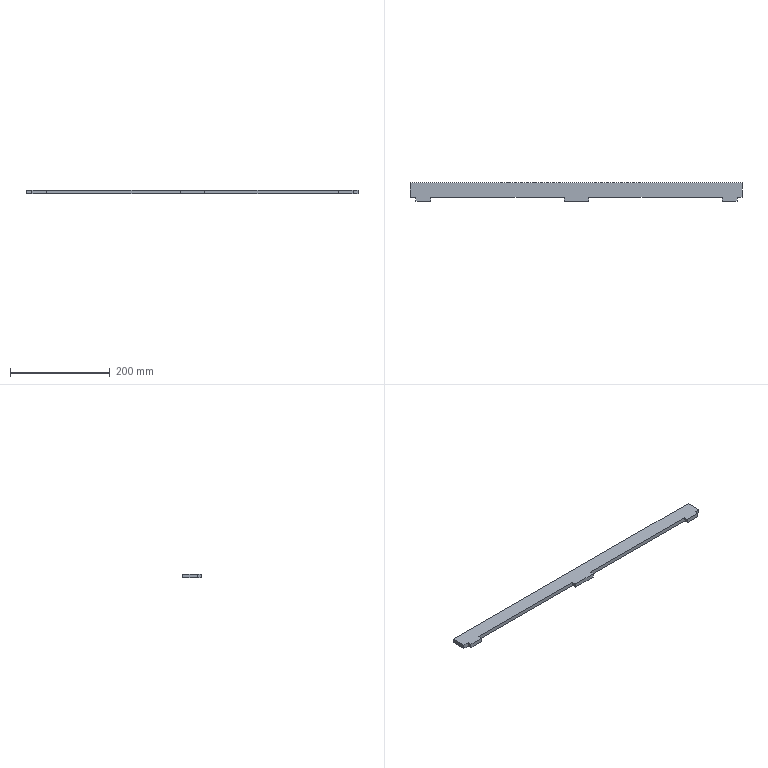Part | SolidWorks | features FlatPattern 1, ICE 1, SMBaseFlange 1, SheetMetal 1 | 1 solid | 18 faces | box 667 x 38 x 8 mm | volume 167120 mm3 | plane 18
STEP:
#1=CARTESIAN_POINT('',(332.5,-15.,-8.));
#2=VERTEX_POINT('',#1);
#3=CARTESIAN_POINT('',(332.5,-15.,0.));
#4=VERTEX_POINT('',#3);
#5=CARTESIAN_POINT('',(332.5,-15.,-8.));
#6=DIRECTION('',(0.,0.,1.));
#7=VECTOR('',#6,1000.);
#8=LINE('',#5,#7);
#9=EDGE_CURVE('',#2,#4,#8,.T.);
#10=ORIENTED_EDGE('',*,*,#9,.T.);
#11=CARTESIAN_POINT('',(322.5,-15.,0.));
#12=VERTEX_POINT('',#11);
#13=CARTESIAN_POINT('',(322.5,-15.,0.));
#14=DIRECTION('',(1.,0.,0.));
#15=VECTOR('',#14,1000.);
#16=LINE('',#13,#15);
#17=EDGE_CURVE('',#12,#4,#16,.T.);
#18=ORIENTED_EDGE('',*,*,#17,.F.);
#19=CARTESIAN_POINT('',(322.5,-15.,-8.));
#20=VERTEX_POINT('',#19);
#21=CARTESIAN_POINT('',(322.5,-15.,-8.));
#22=DIRECTION('',(0.,0.,1.));
#23=VECTOR('',#22,1000.);
#24=LINE('',#21,#23);
#25=EDGE_CURVE('',#20,#12,#24,.T.);
#26=ORIENTED_EDGE('',*,*,#25,.F.);
#27=CARTESIAN_POINT('',(322.5,-15.,-8.));
#28=DIRECTION('',(1.,0.,0.));
#29=VECTOR('',#28,1000.);
#30=LINE('',#27,#29);
#31=EDGE_CURVE('',#20,#2,#30,.T.);
#32=ORIENTED_EDGE('',*,*,#31,.T.);
#33=EDGE_LOOP('',(#10,#18,#26,#32));
#34=FACE_OUTER_BOUND('',#33,.T.);
#35=CARTESIAN_POINT('',(322.5,-15.,-8.));
#36=DIRECTION('',(0.,-1.,0.));
#37=DIRECTION('',(1.,0.,0.));
#38=AXIS2_PLACEMENT_3D('',#35,#36,#37);
#39=PLANE('',#38);
#40=ADVANCED_FACE('',(#34),#39,.T.);
#41=CARTESIAN_POINT('',(322.5,-23.,0.));
#42=VERTEX_POINT('',#41);
#43=CARTESIAN_POINT('',(322.5,-15.,0.));
#44=DIRECTION('',(0.,1.,0.));
#45=VECTOR('',#44,1000.);
#46=LINE('',#43,#45);
#47=EDGE_CURVE('',#42,#12,#46,.T.);
#48=ORIENTED_EDGE('',*,*,#47,.F.);
#49=CARTESIAN_POINT('',(322.5,-23.,-8.));
#50=VERTEX_POINT('',#49);
#51=CARTESIAN_POINT('',(322.5,-23.,-8.));
#52=DIRECTION('',(0.,0.,1.));
#53=VECTOR('',#52,1000.);
#54=LINE('',#51,#53);
#55=EDGE_CURVE('',#50,#42,#54,.T.);
#56=ORIENTED_EDGE('',*,*,#55,.F.);
#57=CARTESIAN_POINT('',(322.5,-15.,-8.));
#58=DIRECTION('',(0.,1.,0.));
#59=VECTOR('',#58,1000.);
#60=LINE('',#57,#59);
#61=EDGE_CURVE('',#50,#20,#60,.T.);
#62=ORIENTED_EDGE('',*,*,#61,.T.);
#63=ORIENTED_EDGE('',*,*,#25,.T.);
#64=EDGE_LOOP('',(#48,#56,#62,#63));
#65=FACE_OUTER_BOUND('',#64,.T.);
#66=CARTESIAN_POINT('',(322.5,-15.,-8.));
#67=DIRECTION('',(1.,0.,0.));
#68=DIRECTION('',(0.,0.,-1.));
#69=AXIS2_PLACEMENT_3D('',#66,#67,#68);
#70=PLANE('',#69);
#71=ADVANCED_FACE('',(#65),#70,.T.);
#72=CARTESIAN_POINT('',(292.5,-23.,0.));
#73=VERTEX_POINT('',#72);
#74=CARTESIAN_POINT('',(322.5,-23.,0.));
#75=DIRECTION('',(1.,0.,0.));
#76=VECTOR('',#75,1000.);
#77=LINE('',#74,#76);
#78=EDGE_CURVE('',#73,#42,#77,.T.);
#79=ORIENTED_EDGE('',*,*,#78,.F.);
#80=CARTESIAN_POINT('',(292.5,-23.,-8.));
#81=VERTEX_POINT('',#80);
#82=CARTESIAN_POINT('',(292.5,-23.,-8.));
#83=DIRECTION('',(0.,0.,1.));
#84=VECTOR('',#83,1000.);
#85=LINE('',#82,#84);
#86=EDGE_CURVE('',#81,#73,#85,.T.);
#87=ORIENTED_EDGE('',*,*,#86,.F.);
#88=CARTESIAN_POINT('',(322.5,-23.,-8.));
#89=DIRECTION('',(1.,0.,0.));
#90=VECTOR('',#89,1000.);
#91=LINE('',#88,#90);
#92=EDGE_CURVE('',#81,#50,#91,.T.);
#93=ORIENTED_EDGE('',*,*,#92,.T.);
#94=ORIENTED_EDGE('',*,*,#55,.T.);
#95=EDGE_LOOP('',(#79,#87,#93,#94));
#96=FACE_OUTER_BOUND('',#95,.T.);
#97=CARTESIAN_POINT('',(322.5,-23.,-8.));
#98=DIRECTION('',(0.,-1.,0.));
#99=DIRECTION('',(1.,0.,0.));
#100=AXIS2_PLACEMENT_3D('',#97,#98,#99);
#101=PLANE('',#100);
#102=ADVANCED_FACE('',(#96),#101,.T.);
#103=CARTESIAN_POINT('',(292.5,-15.,0.));
#104=VERTEX_POINT('',#103);
#105=CARTESIAN_POINT('',(292.5,-23.,0.));
#106=DIRECTION('',(0.,-1.,0.));
#107=VECTOR('',#106,1000.);
#108=LINE('',#105,#107);
#109=EDGE_CURVE('',#104,#73,#108,.T.);
#110=ORIENTED_EDGE('',*,*,#109,.F.);
#111=CARTESIAN_POINT('',(292.5,-15.,-8.));
#112=VERTEX_POINT('',#111);
#113=CARTESIAN_POINT('',(292.5,-15.,-8.));
#114=DIRECTION('',(0.,0.,1.));
#115=VECTOR('',#114,1000.);
#116=LINE('',#113,#115);
#117=EDGE_CURVE('',#112,#104,#116,.T.);
#118=ORIENTED_EDGE('',*,*,#117,.F.);
#119=CARTESIAN_POINT('',(292.5,-23.,-8.));
#120=DIRECTION('',(0.,-1.,0.));
#121=VECTOR('',#120,1000.);
#122=LINE('',#119,#121);
#123=EDGE_CURVE('',#112,#81,#122,.T.);
#124=ORIENTED_EDGE('',*,*,#123,.T.);
#125=ORIENTED_EDGE('',*,*,#86,.T.);
#126=EDGE_LOOP('',(#110,#118,#124,#125));
#127=FACE_OUTER_BOUND('',#126,.T.);
#128=CARTESIAN_POINT('',(292.5,-23.,-8.));
#129=DIRECTION('',(-1.,0.,0.));
#130=DIRECTION('',(0.,0.,1.));
#131=AXIS2_PLACEMENT_3D('',#128,#129,#130);
#132=PLANE('',#131);
#133=ADVANCED_FACE('',(#127),#132,.T.);
#134=CARTESIAN_POINT('',(25.,-15.,0.));
#135=VERTEX_POINT('',#134);
#136=CARTESIAN_POINT('',(25.,-15.,0.));
#137=DIRECTION('',(1.,0.,0.));
#138=VECTOR('',#137,1000.);
#139=LINE('',#136,#138);
#140=EDGE_CURVE('',#135,#104,#139,.T.);
#141=ORIENTED_EDGE('',*,*,#140,.F.);
#142=CARTESIAN_POINT('',(25.,-15.,-8.));
#143=VERTEX_POINT('',#142);
#144=CARTESIAN_POINT('',(25.,-15.,-8.));
#145=DIRECTION('',(0.,0.,1.));
#146=VECTOR('',#145,1000.);
#147=LINE('',#144,#146);
#148=EDGE_CURVE('',#143,#135,#147,.T.);
#149=ORIENTED_EDGE('',*,*,#148,.F.);
#150=CARTESIAN_POINT('',(25.,-15.,-8.));
#151=DIRECTION('',(1.,0.,0.));
#152=VECTOR('',#151,1000.);
#153=LINE('',#150,#152);
#154=EDGE_CURVE('',#143,#112,#153,.T.);
#155=ORIENTED_EDGE('',*,*,#154,.T.);
#156=ORIENTED_EDGE('',*,*,#117,.T.);
#157=EDGE_LOOP('',(#141,#149,#155,#156));
#158=FACE_OUTER_BOUND('',#157,.T.);
#159=CARTESIAN_POINT('',(25.,-15.,-8.));
#160=DIRECTION('',(0.,-1.,0.));
#161=DIRECTION('',(1.,0.,0.));
#162=AXIS2_PLACEMENT_3D('',#159,#160,#161);
#163=PLANE('',#162);
#164=ADVANCED_FACE('',(#158),#163,.T.);
#165=CARTESIAN_POINT('',(25.,-23.,0.));
#166=VERTEX_POINT('',#165);
#167=CARTESIAN_POINT('',(25.,-23.,0.));
#168=DIRECTION('',(0.,1.,0.));
#169=VECTOR('',#168,1000.);
#170=LINE('',#167,#169);
#171=EDGE_CURVE('',#166,#135,#170,.T.);
#172=ORIENTED_EDGE('',*,*,#171,.F.);
#173=CARTESIAN_POINT('',(25.,-23.,-8.));
#174=VERTEX_POINT('',#173);
#175=CARTESIAN_POINT('',(25.,-23.,-8.));
#176=DIRECTION('',(0.,0.,1.));
#177=VECTOR('',#176,1000.);
#178=LINE('',#175,#177);
#179=EDGE_CURVE('',#174,#166,#178,.T.);
#180=ORIENTED_EDGE('',*,*,#179,.F.);
#181=CARTESIAN_POINT('',(25.,-23.,-8.));
#182=DIRECTION('',(0.,1.,0.));
#183=VECTOR('',#182,1000.);
#184=LINE('',#181,#183);
#185=EDGE_CURVE('',#174,#143,#184,.T.);
#186=ORIENTED_EDGE('',*,*,#185,.T.);
#187=ORIENTED_EDGE('',*,*,#148,.T.);
#188=EDGE_LOOP('',(#172,#180,#186,#187));
#189=FACE_OUTER_BOUND('',#188,.T.);
#190=CARTESIAN_POINT('',(25.,-23.,-8.));
#191=DIRECTION('',(1.,0.,0.));
#192=DIRECTION('',(0.,0.,-1.));
#193=AXIS2_PLACEMENT_3D('',#190,#191,#192);
#194=PLANE('',#193);
#195=ADVANCED_FACE('',(#189),#194,.T.);
#196=CARTESIAN_POINT('',(-25.,-23.,0.));
#197=VERTEX_POINT('',#196);
#198=CARTESIAN_POINT('',(-25.,-23.,0.));
#199=DIRECTION('',(1.,0.,0.));
#200=VECTOR('',#199,1000.);
#201=LINE('',#198,#200);
#202=EDGE_CURVE('',#197,#166,#201,.T.);
#203=ORIENTED_EDGE('',*,*,#202,.F.);
#204=CARTESIAN_POINT('',(-25.,-23.,-8.));
#205=VERTEX_POINT('',#204);
#206=CARTESIAN_POINT('',(-25.,-23.,-8.));
#207=DIRECTION('',(0.,0.,1.));
#208=VECTOR('',#207,1000.);
#209=LINE('',#206,#208);
#210=EDGE_CURVE('',#205,#197,#209,.T.);
#211=ORIENTED_EDGE('',*,*,#210,.F.);
#212=CARTESIAN_POINT('',(-25.,-23.,-8.));
#213=DIRECTION('',(1.,0.,0.));
#214=VECTOR('',#213,1000.);
#215=LINE('',#212,#214);
#216=EDGE_CURVE('',#205,#174,#215,.T.);
#217=ORIENTED_EDGE('',*,*,#216,.T.);
#218=ORIENTED_EDGE('',*,*,#179,.T.);
#219=EDGE_LOOP('',(#203,#211,#217,#218));
#220=FACE_OUTER_BOUND('',#219,.T.);
#221=CARTESIAN_POINT('',(-25.,-23.,-8.));
#222=DIRECTION('',(0.,-1.,0.));
#223=DIRECTION('',(1.,0.,0.));
#224=AXIS2_PLACEMENT_3D('',#221,#222,#223);
#225=PLANE('',#224);
#226=ADVANCED_FACE('',(#220),#225,.T.);
#227=CARTESIAN_POINT('',(-25.,-15.,0.));
#228=VERTEX_POINT('',#227);
#229=CARTESIAN_POINT('',(-25.,-15.,0.));
#230=DIRECTION('',(0.,-1.,0.));
#231=VECTOR('',#230,1000.);
#232=LINE('',#229,#231);
#233=EDGE_CURVE('',#228,#197,#232,.T.);
#234=ORIENTED_EDGE('',*,*,#233,.F.);
#235=CARTESIAN_POINT('',(-25.,-15.,-8.));
#236=VERTEX_POINT('',#235);
#237=CARTESIAN_POINT('',(-25.,-15.,-8.));
#238=DIRECTION('',(0.,0.,1.));
#239=VECTOR('',#238,1000.);
#240=LINE('',#237,#239);
#241=EDGE_CURVE('',#236,#228,#240,.T.);
#242=ORIENTED_EDGE('',*,*,#241,.F.);
#243=CARTESIAN_POINT('',(-25.,-15.,-8.));
#244=DIRECTION('',(0.,-1.,0.));
#245=VECTOR('',#244,1000.);
#246=LINE('',#243,#245);
#247=EDGE_CURVE('',#236,#205,#246,.T.);
#248=ORIENTED_EDGE('',*,*,#247,.T.);
#249=ORIENTED_EDGE('',*,*,#210,.T.);
#250=EDGE_LOOP('',(#234,#242,#248,#249));
#251=FACE_OUTER_BOUND('',#250,.T.);
#252=CARTESIAN_POINT('',(-25.,-15.,-8.));
#253=DIRECTION('',(-1.,0.,0.));
#254=DIRECTION('',(0.,0.,1.));
#255=AXIS2_PLACEMENT_3D('',#252,#253,#254);
#256=PLANE('',#255);
#257=ADVANCED_FACE('',(#251),#256,.T.);
#258=CARTESIAN_POINT('',(-292.5,-15.,0.));
#259=VERTEX_POINT('',#258);
#260=CARTESIAN_POINT('',(-292.5,-15.,0.));
#261=DIRECTION('',(1.,0.,0.));
#262=VECTOR('',#261,1000.);
#263=LINE('',#260,#262);
#264=EDGE_CURVE('',#259,#228,#263,.T.);
#265=ORIENTED_EDGE('',*,*,#264,.F.);
#266=CARTESIAN_POINT('',(-292.5,-15.,-8.));
#267=VERTEX_POINT('',#266);
#268=CARTESIAN_POINT('',(-292.5,-15.,-8.));
#269=DIRECTION('',(0.,0.,1.));
#270=VECTOR('',#269,1000.);
#271=LINE('',#268,#270);
#272=EDGE_CURVE('',#267,#259,#271,.T.);
#273=ORIENTED_EDGE('',*,*,#272,.F.);
#274=CARTESIAN_POINT('',(-292.5,-15.,-8.));
#275=DIRECTION('',(1.,0.,0.));
#276=VECTOR('',#275,1000.);
#277=LINE('',#274,#276);
#278=EDGE_CURVE('',#267,#236,#277,.T.);
#279=ORIENTED_EDGE('',*,*,#278,.T.);
#280=ORIENTED_EDGE('',*,*,#241,.T.);
#281=EDGE_LOOP('',(#265,#273,#279,#280));
#282=FACE_OUTER_BOUND('',#281,.T.);
#283=CARTESIAN_POINT('',(-292.5,-15.,-8.));
#284=DIRECTION('',(0.,-1.,0.));
#285=DIRECTION('',(0.,0.,-1.));
#286=AXIS2_PLACEMENT_3D('',#283,#284,#285);
#287=PLANE('',#286);
#288=ADVANCED_FACE('',(#282),#287,.T.);
#289=CARTESIAN_POINT('',(-292.5,-23.,0.));
#290=VERTEX_POINT('',#289);
#291=CARTESIAN_POINT('',(-292.5,-23.,0.));
#292=DIRECTION('',(0.,1.,0.));
#293=VECTOR('',#292,1000.);
#294=LINE('',#291,#293);
#295=EDGE_CURVE('',#290,#259,#294,.T.);
#296=ORIENTED_EDGE('',*,*,#295,.F.);
#297=CARTESIAN_POINT('',(-292.5,-23.,-8.));
#298=VERTEX_POINT('',#297);
#299=CARTESIAN_POINT('',(-292.5,-23.,-8.));
#300=DIRECTION('',(0.,0.,1.));
#301=VECTOR('',#300,1000.);
#302=LINE('',#299,#301);
#303=EDGE_CURVE('',#298,#290,#302,.T.);
#304=ORIENTED_EDGE('',*,*,#303,.F.);
#305=CARTESIAN_POINT('',(-292.5,-23.,-8.));
#306=DIRECTION('',(0.,1.,0.));
#307=VECTOR('',#306,1000.);
#308=LINE('',#305,#307);
#309=EDGE_CURVE('',#298,#267,#308,.T.);
#310=ORIENTED_EDGE('',*,*,#309,.T.);
#311=ORIENTED_EDGE('',*,*,#272,.T.);
#312=EDGE_LOOP('',(#296,#304,#310,#311));
#313=FACE_OUTER_BOUND('',#312,.T.);
#314=CARTESIAN_POINT('',(-292.5,-23.,-8.));
#315=DIRECTION('',(1.,0.,0.));
#316=DIRECTION('',(0.,0.,-1.));
#317=AXIS2_PLACEMENT_3D('',#314,#315,#316);
#318=PLANE('',#317);
#319=ADVANCED_FACE('',(#313),#318,.T.);
#320=CARTESIAN_POINT('',(-322.5,-23.,0.));
#321=VERTEX_POINT('',#320);
#322=CARTESIAN_POINT('',(-322.5,-23.,0.));
#323=DIRECTION('',(1.,0.,0.));
#324=VECTOR('',#323,1000.);
#325=LINE('',#322,#324);
#326=EDGE_CURVE('',#321,#290,#325,.T.);
#327=ORIENTED_EDGE('',*,*,#326,.F.);
#328=CARTESIAN_POINT('',(-322.5,-23.,-8.));
#329=VERTEX_POINT('',#328);
#330=CARTESIAN_POINT('',(-322.5,-23.,-8.));
#331=DIRECTION('',(0.,0.,1.));
#332=VECTOR('',#331,1000.);
#333=LINE('',#330,#332);
#334=EDGE_CURVE('',#329,#321,#333,.T.);
#335=ORIENTED_EDGE('',*,*,#334,.F.);
#336=CARTESIAN_POINT('',(-322.5,-23.,-8.));
#337=DIRECTION('',(1.,0.,0.));
#338=VECTOR('',#337,1000.);
#339=LINE('',#336,#338);
#340=EDGE_CURVE('',#329,#298,#339,.T.);
#341=ORIENTED_EDGE('',*,*,#340,.T.);
#342=ORIENTED_EDGE('',*,*,#303,.T.);
#343=EDGE_LOOP('',(#327,#335,#341,#342));
#344=FACE_OUTER_BOUND('',#343,.T.);
#345=CARTESIAN_POINT('',(-322.5,-23.,-8.));
#346=DIRECTION('',(0.,-1.,0.));
#347=DIRECTION('',(1.,0.,0.));
#348=AXIS2_PLACEMENT_3D('',#345,#346,#347);
#349=PLANE('',#348);
#350=ADVANCED_FACE('',(#344),#349,.T.);
#351=CARTESIAN_POINT('',(-322.5,-15.,0.));
#352=VERTEX_POINT('',#351);
#353=CARTESIAN_POINT('',(-322.5,-15.,0.));
#354=DIRECTION('',(0.,-1.,0.));
#355=VECTOR('',#354,1000.);
#356=LINE('',#353,#355);
#357=EDGE_CURVE('',#352,#321,#356,.T.);
#358=ORIENTED_EDGE('',*,*,#357,.F.);
#359=CARTESIAN_POINT('',(-322.5,-15.,-8.));
#360=VERTEX_POINT('',#359);
#361=CARTESIAN_POINT('',(-322.5,-15.,-8.));
#362=DIRECTION('',(0.,0.,1.));
#363=VECTOR('',#362,1000.);
#364=LINE('',#361,#363);
#365=EDGE_CURVE('',#360,#352,#364,.T.);
#366=ORIENTED_EDGE('',*,*,#365,.F.);
#367=CARTESIAN_POINT('',(-322.5,-15.,-8.));
#368=DIRECTION('',(0.,-1.,0.));
#369=VECTOR('',#368,1000.);
#370=LINE('',#367,#369);
#371=EDGE_CURVE('',#360,#329,#370,.T.);
#372=ORIENTED_EDGE('',*,*,#371,.T.);
#373=ORIENTED_EDGE('',*,*,#334,.T.);
#374=EDGE_LOOP('',(#358,#366,#372,#373));
#375=FACE_OUTER_BOUND('',#374,.T.);
#376=CARTESIAN_POINT('',(-322.5,-15.,-8.));
#377=DIRECTION('',(-1.,0.,0.));
#378=DIRECTION('',(0.,0.,1.));
#379=AXIS2_PLACEMENT_3D('',#376,#377,#378);
#380=PLANE('',#379);
#381=ADVANCED_FACE('',(#375),#380,.T.);
#382=CARTESIAN_POINT('',(-334.5,-15.,-8.));
#383=VERTEX_POINT('',#382);
#384=CARTESIAN_POINT('',(-334.5,-15.,0.));
#385=VERTEX_POINT('',#384);
#386=CARTESIAN_POINT('',(-334.5,-15.,-8.));
#387=DIRECTION('',(0.,0.,1.));
#388=VECTOR('',#387,1000.);
#389=LINE('',#386,#388);
#390=EDGE_CURVE('',#383,#385,#389,.T.);
#391=ORIENTED_EDGE('',*,*,#390,.F.);
#392=CARTESIAN_POINT('',(-357.5,-15.,-8.));
#393=DIRECTION('',(1.,0.,0.));
#394=VECTOR('',#393,1000.);
#395=LINE('',#392,#394);
#396=EDGE_CURVE('',#383,#360,#395,.T.);
#397=ORIENTED_EDGE('',*,*,#396,.T.);
#398=ORIENTED_EDGE('',*,*,#365,.T.);
#399=CARTESIAN_POINT('',(-357.5,-15.,0.));
#400=DIRECTION('',(1.,0.,0.));
#401=VECTOR('',#400,1000.);
#402=LINE('',#399,#401);
#403=EDGE_CURVE('',#385,#352,#402,.T.);
#404=ORIENTED_EDGE('',*,*,#403,.F.);
#405=EDGE_LOOP('',(#391,#397,#398,#404));
#406=FACE_OUTER_BOUND('',#405,.T.);
#407=CARTESIAN_POINT('',(-357.5,-15.,-8.));
#408=DIRECTION('',(0.,-1.,0.));
#409=DIRECTION('',(0.,0.,-1.));
#410=AXIS2_PLACEMENT_3D('',#407,#408,#409);
#411=PLANE('',#410);
#412=ADVANCED_FACE('',(#406),#411,.T.);
#413=CARTESIAN_POINT('',(332.5,15.,-8.));
#414=VERTEX_POINT('',#413);
#415=CARTESIAN_POINT('',(332.5,15.,0.));
#416=VERTEX_POINT('',#415);
#417=CARTESIAN_POINT('',(332.5,15.,-8.));
#418=DIRECTION('',(0.,0.,1.));
#419=VECTOR('',#418,1000.);
#420=LINE('',#417,#419);
#421=EDGE_CURVE('',#414,#416,#420,.T.);
#422=ORIENTED_EDGE('',*,*,#421,.F.);
#423=CARTESIAN_POINT('',(-334.5,15.,-8.));
#424=VERTEX_POINT('',#423);
#425=CARTESIAN_POINT('',(-357.5,15.,-8.));
#426=DIRECTION('',(-1.,0.,0.));
#427=VECTOR('',#426,1000.);
#428=LINE('',#425,#427);
#429=EDGE_CURVE('',#414,#424,#428,.T.);
#430=ORIENTED_EDGE('',*,*,#429,.T.);
#431=CARTESIAN_POINT('',(-334.5,15.,0.));
#432=VERTEX_POINT('',#431);
#433=CARTESIAN_POINT('',(-334.5,15.,-8.));
#434=DIRECTION('',(0.,0.,1.));
#435=VECTOR('',#434,1000.);
#436=LINE('',#433,#435);
#437=EDGE_CURVE('',#424,#432,#436,.T.);
#438=ORIENTED_EDGE('',*,*,#437,.T.);
#439=CARTESIAN_POINT('',(-357.5,15.,0.));
#440=DIRECTION('',(-1.,0.,0.));
#441=VECTOR('',#440,1000.);
#442=LINE('',#439,#441);
#443=EDGE_CURVE('',#416,#432,#442,.T.);
#444=ORIENTED_EDGE('',*,*,#443,.F.);
#445=EDGE_LOOP('',(#422,#430,#438,#444));
#446=FACE_OUTER_BOUND('',#445,.T.);
#447=CARTESIAN_POINT('',(-357.5,15.,-8.));
#448=DIRECTION('',(0.,1.,0.));
#449=DIRECTION('',(0.,0.,1.));
#450=AXIS2_PLACEMENT_3D('',#447,#448,#449);
#451=PLANE('',#450);
#452=ADVANCED_FACE('',(#446),#451,.T.);
#453=CARTESIAN_POINT('',(332.5,-15.,-8.));
#454=DIRECTION('',(0.,-1.,0.));
#455=VECTOR('',#454,1000.);
#456=LINE('',#453,#455);
#457=EDGE_CURVE('',#414,#2,#456,.T.);
#458=ORIENTED_EDGE('',*,*,#457,.T.);
#459=ORIENTED_EDGE('',*,*,#31,.F.);
#460=ORIENTED_EDGE('',*,*,#61,.F.);
#461=ORIENTED_EDGE('',*,*,#92,.F.);
#462=ORIENTED_EDGE('',*,*,#123,.F.);
#463=ORIENTED_EDGE('',*,*,#154,.F.);
#464=ORIENTED_EDGE('',*,*,#185,.F.);
#465=ORIENTED_EDGE('',*,*,#216,.F.);
#466=ORIENTED_EDGE('',*,*,#247,.F.);
#467=ORIENTED_EDGE('',*,*,#278,.F.);
#468=ORIENTED_EDGE('',*,*,#309,.F.);
#469=ORIENTED_EDGE('',*,*,#340,.F.);
#470=ORIENTED_EDGE('',*,*,#371,.F.);
#471=ORIENTED_EDGE('',*,*,#396,.F.);
#472=CARTESIAN_POINT('',(-334.5,-15.,-8.));
#473=DIRECTION('',(0.,1.,0.));
#474=VECTOR('',#473,1000.);
#475=LINE('',#472,#474);
#476=EDGE_CURVE('',#383,#424,#475,.T.);
#477=ORIENTED_EDGE('',*,*,#476,.T.);
#478=ORIENTED_EDGE('',*,*,#429,.F.);
#479=EDGE_LOOP('',(#458,#459,#460,#461,#462,#463,#464,#465,#466,#467,#468,#469,#470,#471,#477,#478));
#480=FACE_OUTER_BOUND('',#479,.T.);
#481=CARTESIAN_POINT('',(0.,0.,-8.));
#482=DIRECTION('',(0.,0.,-1.));
#483=DIRECTION('',(-1.,0.,0.));
#484=AXIS2_PLACEMENT_3D('',#481,#482,#483);
#485=PLANE('',#484);
#486=ADVANCED_FACE('',(#480),#485,.T.);
#487=ORIENTED_EDGE('',*,*,#17,.T.);
#488=CARTESIAN_POINT('',(332.5,-15.,0.));
#489=DIRECTION('',(0.,-1.,0.));
#490=VECTOR('',#489,1000.);
#491=LINE('',#488,#490);
#492=EDGE_CURVE('',#416,#4,#491,.T.);
#493=ORIENTED_EDGE('',*,*,#492,.F.);
#494=ORIENTED_EDGE('',*,*,#443,.T.);
#495=CARTESIAN_POINT('',(-334.5,-15.,0.));
#496=DIRECTION('',(0.,1.,0.));
#497=VECTOR('',#496,1000.);
#498=LINE('',#495,#497);
#499=EDGE_CURVE('',#385,#432,#498,.T.);
#500=ORIENTED_EDGE('',*,*,#499,.F.);
#501=ORIENTED_EDGE('',*,*,#403,.T.);
#502=ORIENTED_EDGE('',*,*,#357,.T.);
#503=ORIENTED_EDGE('',*,*,#326,.T.);
#504=ORIENTED_EDGE('',*,*,#295,.T.);
#505=ORIENTED_EDGE('',*,*,#264,.T.);
#506=ORIENTED_EDGE('',*,*,#233,.T.);
#507=ORIENTED_EDGE('',*,*,#202,.T.);
#508=ORIENTED_EDGE('',*,*,#171,.T.);
#509=ORIENTED_EDGE('',*,*,#140,.T.);
#510=ORIENTED_EDGE('',*,*,#109,.T.);
#511=ORIENTED_EDGE('',*,*,#78,.T.);
#512=ORIENTED_EDGE('',*,*,#47,.T.);
#513=EDGE_LOOP('',(#487,#493,#494,#500,#501,#502,#503,#504,#505,#506,#507,#508,#509,#510,#511,#512));
#514=FACE_OUTER_BOUND('',#513,.T.);
#515=CARTESIAN_POINT('',(0.,0.,0.));
#516=DIRECTION('',(0.,0.,-1.));
#517=DIRECTION('',(-1.,0.,0.));
#518=AXIS2_PLACEMENT_3D('',#515,#516,#517);
#519=PLANE('',#518);
#520=ADVANCED_FACE('',(#514),#519,.F.);
#521=ORIENTED_EDGE('',*,*,#499,.T.);
#522=ORIENTED_EDGE('',*,*,#437,.F.);
#523=ORIENTED_EDGE('',*,*,#476,.F.);
#524=ORIENTED_EDGE('',*,*,#390,.T.);
#525=EDGE_LOOP('',(#521,#522,#523,#524));
#526=FACE_OUTER_BOUND('',#525,.T.);
#527=CARTESIAN_POINT('',(-334.5,-15.,-8.));
#528=DIRECTION('',(1.,0.,0.));
#529=DIRECTION('',(0.,0.,-1.));
#530=AXIS2_PLACEMENT_3D('',#527,#528,#529);
#531=PLANE('',#530);
#532=ADVANCED_FACE('',(#526),#531,.F.);
#533=ORIENTED_EDGE('',*,*,#492,.T.);
#534=ORIENTED_EDGE('',*,*,#9,.F.);
#535=ORIENTED_EDGE('',*,*,#457,.F.);
#536=ORIENTED_EDGE('',*,*,#421,.T.);
#537=EDGE_LOOP('',(#533,#534,#535,#536));
#538=FACE_OUTER_BOUND('',#537,.T.);
#539=CARTESIAN_POINT('',(332.5,-15.,-8.));
#540=DIRECTION('',(-1.,0.,0.));
#541=DIRECTION('',(0.,0.,1.));
#542=AXIS2_PLACEMENT_3D('',#539,#540,#541);
#543=PLANE('',#542);
#544=ADVANCED_FACE('',(#538),#543,.F.);
#545=CLOSED_SHELL('',(#40,#71,#102,#133,#164,#195,#226,#257,#288,#319,#350,#381,#412,#452,#486,#520,#532,#544));
#546=MANIFOLD_SOLID_BREP('',#545);
#547=CARTESIAN_POINT('',(0.,0.,0.));
#548=DIRECTION('',(0.,0.,1.));
#549=DIRECTION('',(1.,0.,0.));
#550=AXIS2_PLACEMENT_3D('',#547,#548,#549);
#551=(LENGTH_UNIT()NAMED_UNIT(*)SI_UNIT(.MILLI.,.METRE.));
#552=UNCERTAINTY_MEASURE_WITH_UNIT(LENGTH_MEASURE(0.00001),#551,'','');
#553=(NAMED_UNIT(*)PLANE_ANGLE_UNIT()SI_UNIT($,.RADIAN.));
#554=(NAMED_UNIT(*)SI_UNIT($,.STERADIAN.)SOLID_ANGLE_UNIT());
#555=(GEOMETRIC_REPRESENTATION_CONTEXT(3)GLOBAL_UNCERTAINTY_ASSIGNED_CONTEXT((#552))GLOBAL_UNIT_ASSIGNED_CONTEXT((#551,#553,#554))REPRESENTATION_CONTEXT('',''));
#556=ADVANCED_BREP_SHAPE_REPRESENTATION('',(#546,#550),#555);